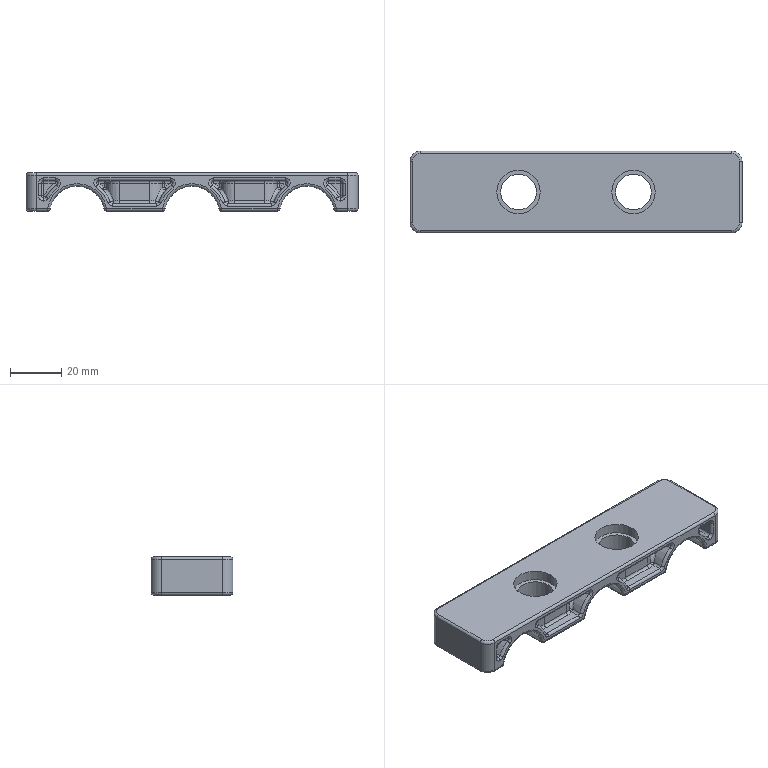Part | SolidWorks | features BaseBody 1 | 1 solid | 336 faces | box 130 x 32 x 15 mm | volume 34645 mm3 | cylinder 138 | torus 87 | sphere 58 | plane 45 | spline 8 | commonest cylinder face diameters 2 x96 27.5 x12 10 x8 17 x8 21.5 x6 8 x4